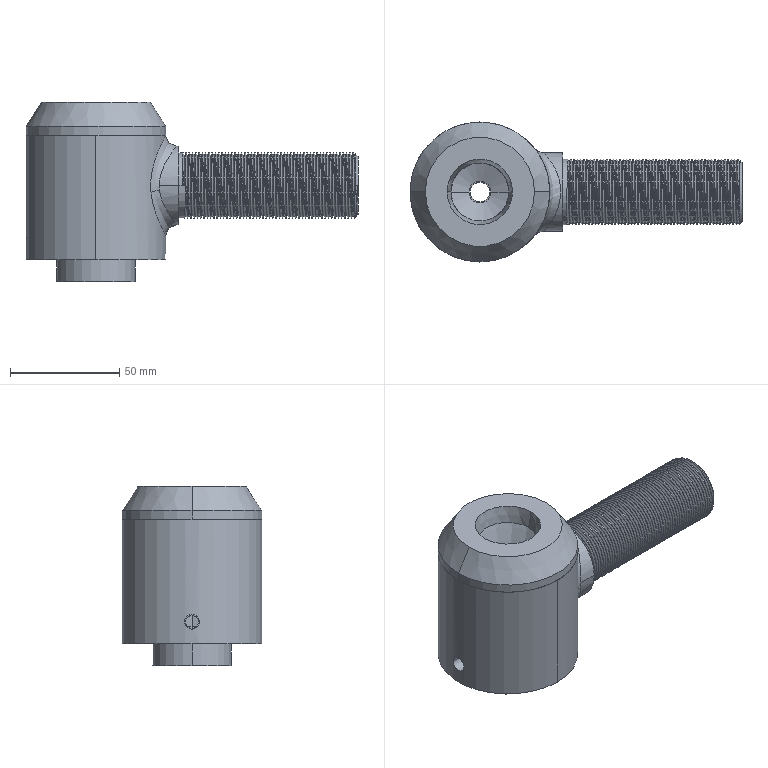Part | SolidWorks | 4 solids | 187 faces | box 152 x 64 x 82 mm | volume 214559 mm3 | cylinder 137 | cone 22 | plane 21 | spline 4 | sphere 3 | commonest cylinder face diameters 30 x106 50 x5 4 x4 36 x4 52 x4 64 x4